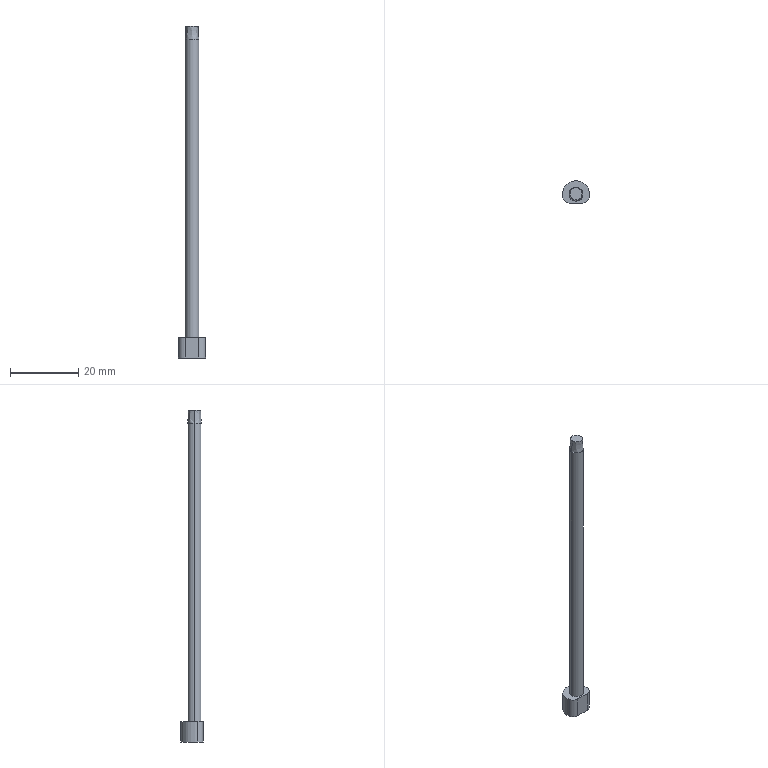Part | Creo | 1 solid | 138 faces | box 8 x 6.5 x 97.252 mm | volume 1399 mm3 | other 95 | plane 35 | cylinder 6 | spline 2 | commonest cylinder face diameters 4 x4 8 x1 8.215 x1